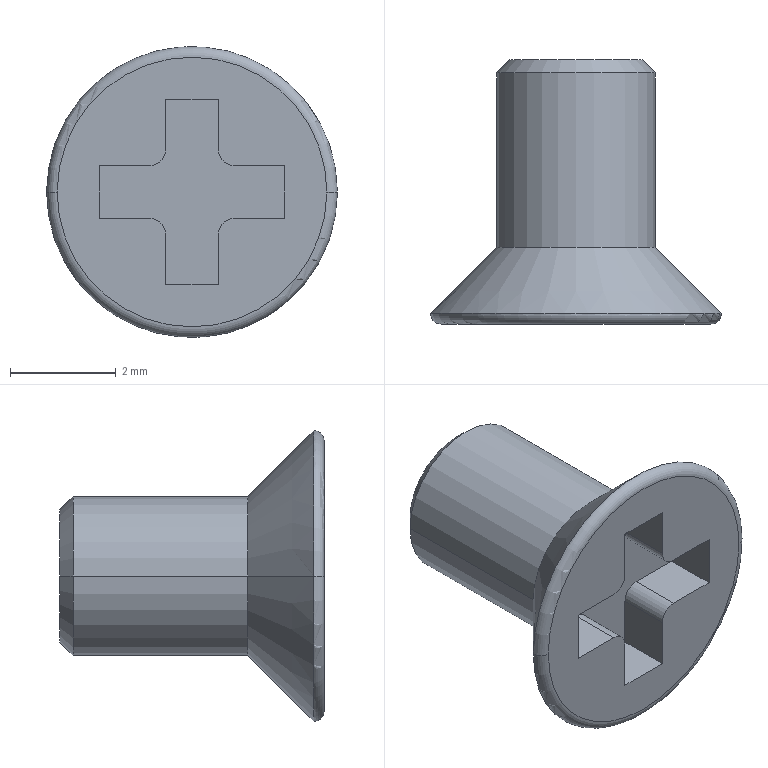Part | STEP file | _X2_751F4E45_X0_MS731-1_X2_8_26 | 1 solid | 27 faces | box 5.5 x 5 x 5.5 mm | volume 41.588 mm3 | plane 15 | cylinder 6 | cone 4 | torus 2 | commonest cylinder face diameters 0.6 x4 3 x2